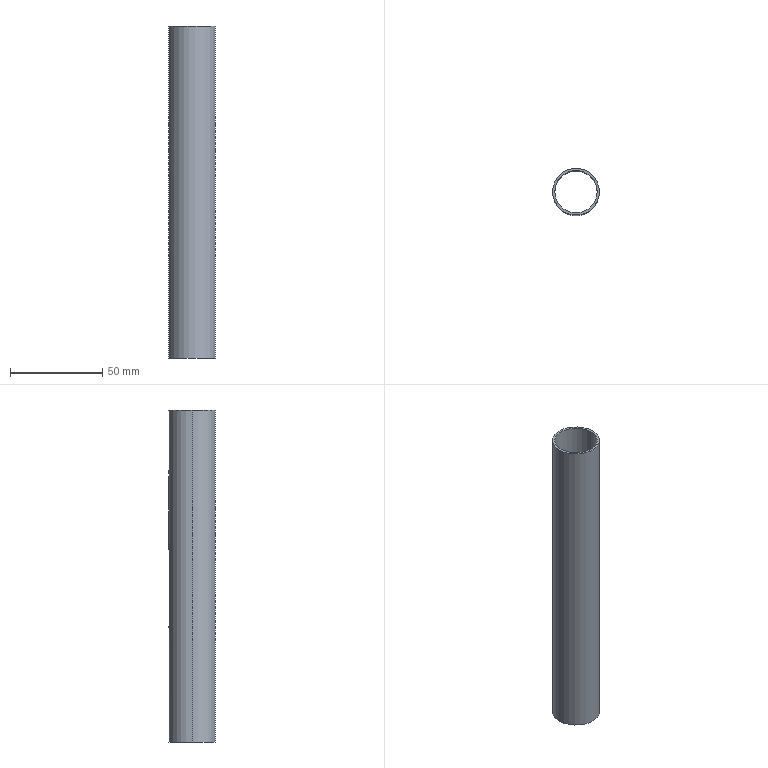Part | STEP file | 31E-01019QY13 | 1 solid | 12 faces | box 25.4 x 25.4 x 180 mm | volume 16074 mm3 | cylinder 8 | plane 4 | commonest cylinder face diameters 4.5 x2 6.5 x2 23 x2 25.4 x2
STEP:
#1=CARTESIAN_POINT('',(-12.7,0.,0.));
#2=VERTEX_POINT('',#1);
#3=CARTESIAN_POINT('',(-12.7,0.,180.));
#4=VERTEX_POINT('',#3);
#5=CARTESIAN_POINT('',(-12.7,0.,90.));
#6=DIRECTION('',(0.,0.,1.));
#7=VECTOR('',#6,1.);
#8=LINE('',#5,#7);
#9=EDGE_CURVE('',#2,#4,#8,.T.);
#10=ORIENTED_EDGE('',*,*,#9,.F.);
#11=CARTESIAN_POINT('',(12.7,0.,0.));
#12=VERTEX_POINT('',#11);
#13=CARTESIAN_POINT('',(0.,0.,0.));
#14=DIRECTION('',(0.,0.,1.));
#15=AXIS2_PLACEMENT_3D('',#13,#14,$);
#16=CIRCLE('',#15,12.7);
#17=EDGE_CURVE('',#2,#12,#16,.T.);
#18=ORIENTED_EDGE('',*,*,#17,.T.);
#19=CARTESIAN_POINT('',(12.7,0.,180.));
#20=VERTEX_POINT('',#19);
#21=CARTESIAN_POINT('',(12.7,0.,90.));
#22=DIRECTION('',(0.,0.,1.));
#23=VECTOR('',#22,1.);
#24=LINE('',#21,#23);
#25=EDGE_CURVE('',#12,#20,#24,.T.);
#26=ORIENTED_EDGE('',*,*,#25,.T.);
#27=CARTESIAN_POINT('',(0.,0.,180.));
#28=DIRECTION('',(0.,0.,1.));
#29=AXIS2_PLACEMENT_3D('',#27,#28,$);
#30=CIRCLE('',#29,12.7);
#31=EDGE_CURVE('',#4,#20,#30,.T.);
#32=ORIENTED_EDGE('',*,*,#31,.F.);
#33=EDGE_LOOP('',(#10,#18,#26,#32));
#34=FACE_OUTER_BOUND('',#33,.T.);
#35=CARTESIAN_POINT('',(0.,0.,90.));
#36=DIRECTION('',(0.,0.,1.));
#37=DIRECTION('',(1.,0.,0.));
#38=AXIS2_PLACEMENT_3D('',#35,#36,#37);
#39=CYLINDRICAL_SURFACE('',#38,12.7);
#40=ADVANCED_FACE('',(#34),#39,.T.);
#41=CARTESIAN_POINT('',(-11.5,0.,180.));
#42=VERTEX_POINT('',#41);
#43=CARTESIAN_POINT('',(11.5,0.,180.));
#44=VERTEX_POINT('',#43);
#45=CARTESIAN_POINT('',(0.,0.,180.));
#46=DIRECTION('',(0.,0.,1.));
#47=AXIS2_PLACEMENT_3D('',#45,#46,$);
#48=CIRCLE('',#47,11.5);
#49=EDGE_CURVE('',#42,#44,#48,.T.);
#50=ORIENTED_EDGE('',*,*,#49,.T.);
#51=CARTESIAN_POINT('',(11.5,0.,0.));
#52=VERTEX_POINT('',#51);
#53=CARTESIAN_POINT('',(11.5,0.,90.));
#54=DIRECTION('',(0.,0.,1.));
#55=VECTOR('',#54,1.);
#56=LINE('',#53,#55);
#57=EDGE_CURVE('',#52,#44,#56,.T.);
#58=ORIENTED_EDGE('',*,*,#57,.F.);
#59=CARTESIAN_POINT('',(-11.5,0.,0.));
#60=VERTEX_POINT('',#59);
#61=CARTESIAN_POINT('',(0.,0.,0.));
#62=DIRECTION('',(0.,0.,1.));
#63=AXIS2_PLACEMENT_3D('',#61,#62,$);
#64=CIRCLE('',#63,11.5);
#65=EDGE_CURVE('',#60,#52,#64,.T.);
#66=ORIENTED_EDGE('',*,*,#65,.F.);
#67=CARTESIAN_POINT('',(-11.5,0.,90.));
#68=DIRECTION('',(0.,0.,1.));
#69=VECTOR('',#68,1.);
#70=LINE('',#67,#69);
#71=EDGE_CURVE('',#60,#42,#70,.T.);
#72=ORIENTED_EDGE('',*,*,#71,.T.);
#73=EDGE_LOOP('',(#50,#58,#66,#72));
#74=FACE_OUTER_BOUND('',#73,.T.);
#75=CARTESIAN_POINT('',(0.,0.,90.));
#76=DIRECTION('',(0.,0.,1.));
#77=DIRECTION('',(1.,0.,0.));
#78=AXIS2_PLACEMENT_3D('',#75,#76,#77);
#79=CYLINDRICAL_SURFACE('',#78,11.5);
#80=ADVANCED_FACE('',(#74),#79,.F.);
#81=ORIENTED_EDGE('',*,*,#17,.F.);
#82=CARTESIAN_POINT('',(0.,0.,0.));
#83=DIRECTION('',(0.,0.,1.));
#84=AXIS2_PLACEMENT_3D('',#82,#83,$);
#85=CIRCLE('',#84,12.7);
#86=EDGE_CURVE('',#12,#2,#85,.T.);
#87=ORIENTED_EDGE('',*,*,#86,.F.);
#88=EDGE_LOOP('',(#81,#87));
#89=FACE_OUTER_BOUND('',#88,.T.);
#90=CARTESIAN_POINT('',(0.,0.,0.));
#91=DIRECTION('',(0.,0.,1.));
#92=AXIS2_PLACEMENT_3D('',#90,#91,$);
#93=CIRCLE('',#92,11.5);
#94=EDGE_CURVE('',#52,#60,#93,.T.);
#95=ORIENTED_EDGE('',*,*,#94,.T.);
#96=ORIENTED_EDGE('',*,*,#65,.T.);
#97=EDGE_LOOP('',(#95,#96));
#98=FACE_BOUND('',#97,.T.);
#99=CARTESIAN_POINT('',(0.,0.,0.));
#100=DIRECTION('',(0.,0.,1.));
#101=DIRECTION('',(1.,0.,0.));
#102=AXIS2_PLACEMENT_3D('',#99,#100,#101);
#103=PLANE('',#102);
#104=ADVANCED_FACE('',(#89,#98),#103,.F.);
#105=CARTESIAN_POINT('',(0.,0.,180.));
#106=DIRECTION('',(0.,0.,1.));
#107=AXIS2_PLACEMENT_3D('',#105,#106,$);
#108=CIRCLE('',#107,12.7);
#109=EDGE_CURVE('',#20,#4,#108,.T.);
#110=ORIENTED_EDGE('',*,*,#109,.T.);
#111=ORIENTED_EDGE('',*,*,#31,.T.);
#112=EDGE_LOOP('',(#110,#111));
#113=FACE_OUTER_BOUND('',#112,.T.);
#114=ORIENTED_EDGE('',*,*,#49,.F.);
#115=CARTESIAN_POINT('',(0.,0.,180.));
#116=DIRECTION('',(0.,0.,1.));
#117=AXIS2_PLACEMENT_3D('',#115,#116,$);
#118=CIRCLE('',#117,11.5);
#119=EDGE_CURVE('',#44,#42,#118,.T.);
#120=ORIENTED_EDGE('',*,*,#119,.F.);
#121=EDGE_LOOP('',(#114,#120));
#122=FACE_BOUND('',#121,.T.);
#123=CARTESIAN_POINT('',(0.,0.,180.));
#124=DIRECTION('',(0.,0.,1.));
#125=DIRECTION('',(1.,0.,0.));
#126=AXIS2_PLACEMENT_3D('',#123,#124,#125);
#127=PLANE('',#126);
#128=ADVANCED_FACE('',(#113,#122),#127,.T.);
#129=ORIENTED_EDGE('',*,*,#119,.T.);
#130=ORIENTED_EDGE('',*,*,#71,.F.);
#131=ORIENTED_EDGE('',*,*,#94,.F.);
#132=ORIENTED_EDGE('',*,*,#57,.T.);
#133=EDGE_LOOP('',(#129,#130,#131,#132));
#134=FACE_OUTER_BOUND('',#133,.T.);
#135=CARTESIAN_POINT('',(0.,11.5,147.25));
#136=VERTEX_POINT('',#135);
#137=CARTESIAN_POINT('',(0.,11.5,142.75));
#138=VERTEX_POINT('',#137);
#139=CARTESIAN_POINT('',(0.,11.5,147.25));
#140=CARTESIAN_POINT('',(0.722,11.5,147.25));
#141=CARTESIAN_POINT('',(1.444,11.443,146.96));
#142=CARTESIAN_POINT('',(2.003,11.327,146.385));
#143=CARTESIAN_POINT('',(2.528,11.222,144.951));
#144=CARTESIAN_POINT('',(1.939,11.34,143.552));
#145=CARTESIAN_POINT('',(1.39,11.447,143.018));
#146=CARTESIAN_POINT('',(0.6951,11.5,142.75));
#147=CARTESIAN_POINT('',(0.,11.5,142.75));
#148=B_SPLINE_CURVE_WITH_KNOTS('',5,(#139,#140,#141,#142,#143,#144,#145,#146,#147),.UNSPECIFIED.,.F.,.U.,(6,3,6),(0.,5.105,10.02),.UNSPECIFIED.);
#149=EDGE_CURVE('',#136,#138,#148,.T.);
#150=ORIENTED_EDGE('',*,*,#149,.T.);
#151=CARTESIAN_POINT('',(0.,11.5,142.75));
#152=CARTESIAN_POINT('',(-0.722,11.5,142.75));
#153=CARTESIAN_POINT('',(-1.444,11.443,143.04));
#154=CARTESIAN_POINT('',(-2.003,11.327,143.615));
#155=CARTESIAN_POINT('',(-2.528,11.222,145.049));
#156=CARTESIAN_POINT('',(-1.939,11.34,146.448));
#157=CARTESIAN_POINT('',(-1.39,11.447,146.982));
#158=CARTESIAN_POINT('',(-0.6951,11.5,147.25));
#159=CARTESIAN_POINT('',(0.,11.5,147.25));
#160=B_SPLINE_CURVE_WITH_KNOTS('',5,(#151,#152,#153,#154,#155,#156,#157,#158,#159),.UNSPECIFIED.,.F.,.U.,(6,3,6),(0.,5.105,10.02),.UNSPECIFIED.);
#161=EDGE_CURVE('',#138,#136,#160,.T.);
#162=ORIENTED_EDGE('',*,*,#161,.T.);
#163=EDGE_LOOP('',(#150,#162));
#164=FACE_BOUND('',#163,.T.);
#165=CARTESIAN_POINT('',(3.25,11.031,65.25));
#166=VERTEX_POINT('',#165);
#167=CARTESIAN_POINT('',(3.25,11.031,101.75));
#168=VERTEX_POINT('',#167);
#169=CARTESIAN_POINT('',(3.25,11.031,90.));
#170=DIRECTION('',(0.,0.,1.));
#171=VECTOR('',#170,1.);
#172=LINE('',#169,#171);
#173=EDGE_CURVE('',#166,#168,#172,.T.);
#174=ORIENTED_EDGE('',*,*,#173,.F.);
#175=CARTESIAN_POINT('',(-3.25,11.031,65.25));
#176=VERTEX_POINT('',#175);
#177=CARTESIAN_POINT('',(3.25,11.031,65.25));
#178=CARTESIAN_POINT('',(3.25,11.031,64.668));
#179=CARTESIAN_POINT('',(3.12,11.07,64.087));
#180=CARTESIAN_POINT('',(2.86,11.146,63.549));
#181=CARTESIAN_POINT('',(2.267,11.291,62.803));
#182=CARTESIAN_POINT('',(1.462,11.413,62.314));
#183=CARTESIAN_POINT('',(1.129,11.452,62.171));
#184=CARTESIAN_POINT('',(0.2075,11.523,61.917));
#185=CARTESIAN_POINT('',(-0.7628,11.499,62.006));
#186=CARTESIAN_POINT('',(-1.34,11.441,62.201));
#187=CARTESIAN_POINT('',(-2.301,11.285,62.792));
#188=CARTESIAN_POINT('',(-2.936,11.124,63.716));
#189=CARTESIAN_POINT('',(-3.145,11.062,64.206));
#190=CARTESIAN_POINT('',(-3.25,11.031,64.728));
#191=CARTESIAN_POINT('',(-3.25,11.031,65.25));
#192=B_SPLINE_CURVE_WITH_KNOTS('',5,(#177,#178,#179,#180,#181,#182,#183,#184,#185,#186,#187,#188,#189,#190,#191),.UNSPECIFIED.,.F.,.U.,(6,3,3,3,6),(0.,4.113,6.656,10.823,14.513),.UNSPECIFIED.);
#193=EDGE_CURVE('',#166,#176,#192,.T.);
#194=ORIENTED_EDGE('',*,*,#193,.T.);
#195=CARTESIAN_POINT('',(-3.25,11.031,101.75));
#196=VERTEX_POINT('',#195);
#197=CARTESIAN_POINT('',(-3.25,11.031,90.));
#198=DIRECTION('',(0.,0.,1.));
#199=VECTOR('',#198,1.);
#200=LINE('',#197,#199);
#201=EDGE_CURVE('',#196,#176,#200,.F.);
#202=ORIENTED_EDGE('',*,*,#201,.F.);
#203=CARTESIAN_POINT('',(3.25,11.031,101.75));
#204=CARTESIAN_POINT('',(3.25,11.031,102.332));
#205=CARTESIAN_POINT('',(3.12,11.07,102.913));
#206=CARTESIAN_POINT('',(2.86,11.146,103.451));
#207=CARTESIAN_POINT('',(2.267,11.291,104.197));
#208=CARTESIAN_POINT('',(1.462,11.413,104.686));
#209=CARTESIAN_POINT('',(1.129,11.452,104.829));
#210=CARTESIAN_POINT('',(0.2075,11.523,105.083));
#211=CARTESIAN_POINT('',(-0.7628,11.499,104.994));
#212=CARTESIAN_POINT('',(-1.34,11.441,104.799));
#213=CARTESIAN_POINT('',(-2.301,11.285,104.208));
#214=CARTESIAN_POINT('',(-2.936,11.124,103.284));
#215=CARTESIAN_POINT('',(-3.145,11.062,102.794));
#216=CARTESIAN_POINT('',(-3.25,11.031,102.272));
#217=CARTESIAN_POINT('',(-3.25,11.031,101.75));
#218=B_SPLINE_CURVE_WITH_KNOTS('',5,(#203,#204,#205,#206,#207,#208,#209,#210,#211,#212,#213,#214,#215,#216,#217),.UNSPECIFIED.,.F.,.U.,(6,3,3,3,6),(0.,4.113,6.656,10.823,14.513),.UNSPECIFIED.);
#219=EDGE_CURVE('',#168,#196,#218,.T.);
#220=ORIENTED_EDGE('',*,*,#219,.F.);
#221=EDGE_LOOP('',(#174,#194,#202,#220));
#222=FACE_BOUND('',#221,.T.);
#223=ADVANCED_FACE('',(#134,#164,#222),#79,.F.);
#224=ORIENTED_EDGE('',*,*,#25,.F.);
#225=ORIENTED_EDGE('',*,*,#86,.T.);
#226=ORIENTED_EDGE('',*,*,#9,.T.);
#227=ORIENTED_EDGE('',*,*,#109,.F.);
#228=EDGE_LOOP('',(#224,#225,#226,#227));
#229=FACE_OUTER_BOUND('',#228,.T.);
#230=CARTESIAN_POINT('',(0.,12.7,142.75));
#231=VERTEX_POINT('',#230);
#232=CARTESIAN_POINT('',(0.,12.7,147.25));
#233=VERTEX_POINT('',#232);
#234=CARTESIAN_POINT('',(0.,12.7,142.75));
#235=CARTESIAN_POINT('',(-0.7217,12.7,142.75));
#236=CARTESIAN_POINT('',(-1.443,12.649,143.039));
#237=CARTESIAN_POINT('',(-2.003,12.544,143.616));
#238=CARTESIAN_POINT('',(-2.528,12.449,145.049));
#239=CARTESIAN_POINT('',(-1.939,12.555,146.448));
#240=CARTESIAN_POINT('',(-1.39,12.652,146.982));
#241=CARTESIAN_POINT('',(-0.6948,12.7,147.25));
#242=CARTESIAN_POINT('',(0.,12.7,147.25));
#243=B_SPLINE_CURVE_WITH_KNOTS('',5,(#234,#235,#236,#237,#238,#239,#240,#241,#242),.UNSPECIFIED.,.F.,.U.,(6,3,6),(0.,5.103,10.016),.UNSPECIFIED.);
#244=EDGE_CURVE('',#231,#233,#243,.T.);
#245=ORIENTED_EDGE('',*,*,#244,.F.);
#246=CARTESIAN_POINT('',(0.,12.7,147.25));
#247=CARTESIAN_POINT('',(0.7217,12.7,147.25));
#248=CARTESIAN_POINT('',(1.443,12.649,146.961));
#249=CARTESIAN_POINT('',(2.003,12.544,146.384));
#250=CARTESIAN_POINT('',(2.528,12.449,144.951));
#251=CARTESIAN_POINT('',(1.939,12.555,143.552));
#252=CARTESIAN_POINT('',(1.39,12.652,143.018));
#253=CARTESIAN_POINT('',(0.6948,12.7,142.75));
#254=CARTESIAN_POINT('',(0.,12.7,142.75));
#255=B_SPLINE_CURVE_WITH_KNOTS('',5,(#246,#247,#248,#249,#250,#251,#252,#253,#254),.UNSPECIFIED.,.F.,.U.,(6,3,6),(0.,5.103,10.016),.UNSPECIFIED.);
#256=EDGE_CURVE('',#233,#231,#255,.T.);
#257=ORIENTED_EDGE('',*,*,#256,.F.);
#258=EDGE_LOOP('',(#245,#257));
#259=FACE_BOUND('',#258,.T.);
#260=CARTESIAN_POINT('',(-3.25,12.277,101.75));
#261=VERTEX_POINT('',#260);
#262=CARTESIAN_POINT('',(3.25,12.277,101.75));
#263=VERTEX_POINT('',#262);
#264=CARTESIAN_POINT('',(-3.25,12.277,101.75));
#265=CARTESIAN_POINT('',(-3.25,12.277,102.455));
#266=CARTESIAN_POINT('',(-3.059,12.328,103.159));
#267=CARTESIAN_POINT('',(-2.679,12.429,103.787));
#268=CARTESIAN_POINT('',(-1.888,12.583,104.534));
#269=CARTESIAN_POINT('',(-0.8884,12.676,104.907));
#270=CARTESIAN_POINT('',(-0.5367,12.696,104.985));
#271=CARTESIAN_POINT('',(0.4785,12.717,105.068));
#272=CARTESIAN_POINT('',(1.471,12.639,104.76));
#273=CARTESIAN_POINT('',(2.044,12.549,104.403));
#274=CARTESIAN_POINT('',(2.742,12.406,103.672));
#275=CARTESIAN_POINT('',(3.119,12.312,102.753));
#276=CARTESIAN_POINT('',(3.206,12.289,102.424));
#277=CARTESIAN_POINT('',(3.25,12.277,102.087));
#278=CARTESIAN_POINT('',(3.25,12.277,101.75));
#279=B_SPLINE_CURVE_WITH_KNOTS('',5,(#264,#265,#266,#267,#268,#269,#270,#271,#272,#273,#274,#275,#276,#277,#278),.UNSPECIFIED.,.F.,.U.,(6,3,3,3,6),(0.,4.982,7.501,12.115,14.499),.UNSPECIFIED.);
#280=EDGE_CURVE('',#261,#263,#279,.T.);
#281=ORIENTED_EDGE('',*,*,#280,.F.);
#282=CARTESIAN_POINT('',(-3.25,12.277,65.25));
#283=VERTEX_POINT('',#282);
#284=CARTESIAN_POINT('',(-3.25,12.277,90.));
#285=DIRECTION('',(0.,0.,1.));
#286=VECTOR('',#285,1.);
#287=LINE('',#284,#286);
#288=EDGE_CURVE('',#261,#283,#287,.F.);
#289=ORIENTED_EDGE('',*,*,#288,.T.);
#290=CARTESIAN_POINT('',(3.25,12.277,65.25));
#291=VERTEX_POINT('',#290);
#292=CARTESIAN_POINT('',(3.25,12.277,65.25));
#293=CARTESIAN_POINT('',(3.25,12.277,64.545));
#294=CARTESIAN_POINT('',(3.059,12.328,63.841));
#295=CARTESIAN_POINT('',(2.679,12.429,63.213));
#296=CARTESIAN_POINT('',(1.888,12.583,62.466));
#297=CARTESIAN_POINT('',(0.8884,12.676,62.093));
#298=CARTESIAN_POINT('',(0.5367,12.696,62.015));
#299=CARTESIAN_POINT('',(-0.4785,12.717,61.932));
#300=CARTESIAN_POINT('',(-1.471,12.639,62.24));
#301=CARTESIAN_POINT('',(-2.044,12.549,62.597));
#302=CARTESIAN_POINT('',(-2.742,12.406,63.328));
#303=CARTESIAN_POINT('',(-3.119,12.312,64.247));
#304=CARTESIAN_POINT('',(-3.206,12.289,64.576));
#305=CARTESIAN_POINT('',(-3.25,12.277,64.913));
#306=CARTESIAN_POINT('',(-3.25,12.277,65.25));
#307=B_SPLINE_CURVE_WITH_KNOTS('',5,(#292,#293,#294,#295,#296,#297,#298,#299,#300,#301,#302,#303,#304,#305,#306),.UNSPECIFIED.,.F.,.U.,(6,3,3,3,6),(0.,4.982,7.501,12.115,14.499),.UNSPECIFIED.);
#308=EDGE_CURVE('',#291,#283,#307,.T.);
#309=ORIENTED_EDGE('',*,*,#308,.F.);
#310=CARTESIAN_POINT('',(3.25,12.277,90.));
#311=DIRECTION('',(0.,0.,1.));
#312=VECTOR('',#311,1.);
#313=LINE('',#310,#312);
#314=EDGE_CURVE('',#291,#263,#313,.T.);
#315=ORIENTED_EDGE('',*,*,#314,.T.);
#316=EDGE_LOOP('',(#281,#289,#309,#315));
#317=FACE_BOUND('',#316,.T.);
#318=ADVANCED_FACE('',(#229,#259,#317),#39,.T.);
#319=ORIENTED_EDGE('',*,*,#173,.T.);
#320=CARTESIAN_POINT('',(3.25,11.654,101.75));
#321=DIRECTION('',(0.,1.,0.));
#322=VECTOR('',#321,1.);
#323=LINE('',#320,#322);
#324=EDGE_CURVE('',#168,#263,#323,.T.);
#325=ORIENTED_EDGE('',*,*,#324,.T.);
#326=ORIENTED_EDGE('',*,*,#314,.F.);
#327=CARTESIAN_POINT('',(3.25,11.654,65.25));
#328=DIRECTION('',(0.,1.,0.));
#329=VECTOR('',#328,1.);
#330=LINE('',#327,#329);
#331=EDGE_CURVE('',#166,#291,#330,.T.);
#332=ORIENTED_EDGE('',*,*,#331,.F.);
#333=EDGE_LOOP('',(#319,#325,#326,#332));
#334=FACE_OUTER_BOUND('',#333,.T.);
#335=CARTESIAN_POINT('',(3.25,0.,65.25));
#336=DIRECTION('',(-1.,0.,0.));
#337=DIRECTION('',(0.,0.,1.));
#338=AXIS2_PLACEMENT_3D('',#335,#336,#337);
#339=PLANE('',#338);
#340=ADVANCED_FACE('',(#334),#339,.T.);
#341=CARTESIAN_POINT('',(-3.25,90.,101.75));
#342=DIRECTION('',(0.,1.,0.));
#343=VECTOR('',#342,1.);
#344=LINE('',#341,#343);
#345=EDGE_CURVE('',#196,#261,#344,.T.);
#346=ORIENTED_EDGE('',*,*,#345,.T.);
#347=ORIENTED_EDGE('',*,*,#280,.T.);
#348=ORIENTED_EDGE('',*,*,#324,.F.);
#349=ORIENTED_EDGE('',*,*,#219,.T.);
#350=EDGE_LOOP('',(#346,#347,#348,#349));
#351=FACE_OUTER_BOUND('',#350,.T.);
#352=CARTESIAN_POINT('',(0.,90.,101.75));
#353=DIRECTION('',(0.,1.,0.));
#354=DIRECTION('',(-1.,0.,0.));
#355=AXIS2_PLACEMENT_3D('',#352,#353,#354);
#356=CYLINDRICAL_SURFACE('',#355,3.25);
#357=ADVANCED_FACE('',(#351),#356,.F.);
#358=ORIENTED_EDGE('',*,*,#331,.T.);
#359=ORIENTED_EDGE('',*,*,#308,.T.);
#360=CARTESIAN_POINT('',(-3.25,90.,65.25));
#361=DIRECTION('',(0.,1.,0.));
#362=VECTOR('',#361,1.);
#363=LINE('',#360,#362);
#364=EDGE_CURVE('',#176,#283,#363,.T.);
#365=ORIENTED_EDGE('',*,*,#364,.F.);
#366=ORIENTED_EDGE('',*,*,#193,.F.);
#367=EDGE_LOOP('',(#358,#359,#365,#366));
#368=FACE_OUTER_BOUND('',#367,.T.);
#369=CARTESIAN_POINT('',(0.,90.,65.25));
#370=DIRECTION('',(0.,1.,0.));
#371=DIRECTION('',(1.,0.,0.));
#372=AXIS2_PLACEMENT_3D('',#369,#370,#371);
#373=CYLINDRICAL_SURFACE('',#372,3.25);
#374=ADVANCED_FACE('',(#368),#373,.F.);
#375=ORIENTED_EDGE('',*,*,#201,.T.);
#376=ORIENTED_EDGE('',*,*,#364,.T.);
#377=ORIENTED_EDGE('',*,*,#288,.F.);
#378=ORIENTED_EDGE('',*,*,#345,.F.);
#379=EDGE_LOOP('',(#375,#376,#377,#378));
#380=FACE_OUTER_BOUND('',#379,.T.);
#381=CARTESIAN_POINT('',(-3.25,0.,101.75));
#382=DIRECTION('',(1.,0.,0.));
#383=DIRECTION('',(0.,0.,-1.));
#384=AXIS2_PLACEMENT_3D('',#381,#382,#383);
#385=PLANE('',#384);
#386=ADVANCED_FACE('',(#380),#385,.T.);
#387=CARTESIAN_POINT('',(0.,90.,147.25));
#388=DIRECTION('',(0.,1.,0.));
#389=VECTOR('',#388,1.);
#390=LINE('',#387,#389);
#391=EDGE_CURVE('',#136,#233,#390,.T.);
#392=ORIENTED_EDGE('',*,*,#391,.T.);
#393=ORIENTED_EDGE('',*,*,#256,.T.);
#394=CARTESIAN_POINT('',(0.,90.,142.75));
#395=DIRECTION('',(0.,1.,0.));
#396=VECTOR('',#395,1.);
#397=LINE('',#394,#396);
#398=EDGE_CURVE('',#138,#231,#397,.T.);
#399=ORIENTED_EDGE('',*,*,#398,.F.);
#400=ORIENTED_EDGE('',*,*,#149,.F.);
#401=EDGE_LOOP('',(#392,#393,#399,#400));
#402=FACE_OUTER_BOUND('',#401,.T.);
#403=CARTESIAN_POINT('',(0.,90.,145.));
#404=DIRECTION('',(0.,1.,0.));
#405=DIRECTION('',(0.,0.,-1.));
#406=AXIS2_PLACEMENT_3D('',#403,#404,#405);
#407=CYLINDRICAL_SURFACE('',#406,2.25);
#408=ADVANCED_FACE('',(#402),#407,.F.);
#409=ORIENTED_EDGE('',*,*,#398,.T.);
#410=ORIENTED_EDGE('',*,*,#244,.T.);
#411=ORIENTED_EDGE('',*,*,#391,.F.);
#412=ORIENTED_EDGE('',*,*,#161,.F.);
#413=EDGE_LOOP('',(#409,#410,#411,#412));
#414=FACE_OUTER_BOUND('',#413,.T.);
#415=ADVANCED_FACE('',(#414),#407,.F.);
#416=CLOSED_SHELL('',(#40,#80,#104,#128,#223,#318,#340,#357,#374,#386,#408,#415));
#417=MANIFOLD_SOLID_BREP('',#416);
#418=(LENGTH_UNIT()NAMED_UNIT(*)SI_UNIT(.MILLI.,.METRE.));
#419=UNCERTAINTY_MEASURE_WITH_UNIT(LENGTH_MEASURE(0.005),#418,'','');
#420=(NAMED_UNIT(*)PLANE_ANGLE_UNIT()SI_UNIT($,.RADIAN.));
#421=(NAMED_UNIT(*)SI_UNIT($,.STERADIAN.)SOLID_ANGLE_UNIT());
#422=(GEOMETRIC_REPRESENTATION_CONTEXT(3)GLOBAL_UNCERTAINTY_ASSIGNED_CONTEXT((#419))GLOBAL_UNIT_ASSIGNED_CONTEXT((#418,#420,#421))REPRESENTATION_CONTEXT('',''));
#423=ADVANCED_BREP_SHAPE_REPRESENTATION('',(#417),#422);